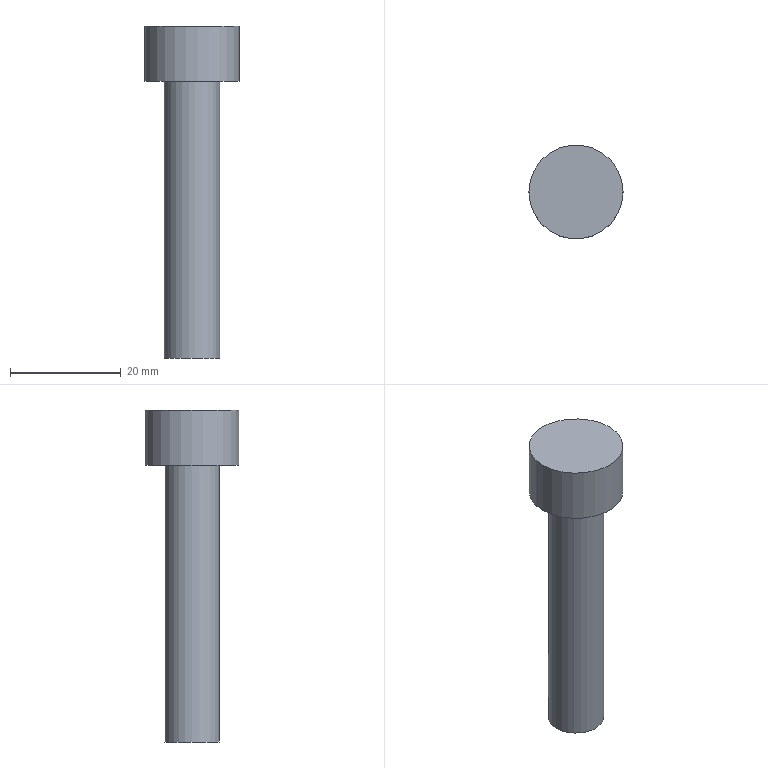Part | NX | features solid 2 | 1 solid | 5 faces | box 17 x 17 x 60 mm | volume 6197 mm3 | plane 3 | cylinder 2 | commonest cylinder face diameters 10 x1 17 x1
STEP:
#1=CARTESIAN_POINT('',(-5.,447.,-123.));
#2=VERTEX_POINT('',#1);
#3=CARTESIAN_POINT('',(0.,447.,-123.));
#4=DIRECTION('',(0.,0.,-1.));
#5=DIRECTION('',(-1.,0.,0.));
#6=AXIS2_PLACEMENT_3D('',#3,#4,#5);
#7=CIRCLE('',#6,5.);
#8=EDGE_CURVE('',#2,#2,#7,.T.);
#9=ORIENTED_EDGE('',*,*,#8,.T.);
#10=EDGE_LOOP('',(#9));
#11=FACE_BOUND('',#10,.T.);
#12=CARTESIAN_POINT('',(0.,447.,-123.));
#13=DIRECTION('',(0.,0.,-1.));
#14=DIRECTION('',(-1.,0.,0.));
#15=AXIS2_PLACEMENT_3D('',#12,#13,#14);
#16=PLANE('',#15);
#17=ADVANCED_FACE('',(#11),#16,.T.);
#18=CARTESIAN_POINT('',(-5.,447.,-73.));
#19=VERTEX_POINT('',#18);
#20=CARTESIAN_POINT('',(0.,447.,-73.));
#21=DIRECTION('',(0.,0.,-1.));
#22=DIRECTION('',(-1.,0.,0.));
#23=AXIS2_PLACEMENT_3D('',#20,#21,#22);
#24=CIRCLE('',#23,5.);
#25=EDGE_CURVE('',#19,#19,#24,.F.);
#26=ORIENTED_EDGE('',*,*,#25,.F.);
#27=EDGE_LOOP('',(#26));
#28=FACE_BOUND('',#27,.T.);
#29=ORIENTED_EDGE('',*,*,#8,.F.);
#30=EDGE_LOOP('',(#29));
#31=FACE_BOUND('',#30,.T.);
#32=CARTESIAN_POINT('',(0.,447.,-83.));
#33=DIRECTION('',(0.,0.,-1.));
#34=DIRECTION('',(-1.,0.,0.));
#35=AXIS2_PLACEMENT_3D('',#32,#33,#34);
#36=CYLINDRICAL_SURFACE('',#35,5.);
#37=ADVANCED_FACE('',(#28,#31),#36,.T.);
#38=CARTESIAN_POINT('',(-8.5,447.,-63.));
#39=VERTEX_POINT('',#38);
#40=CARTESIAN_POINT('',(0.,447.,-63.));
#41=DIRECTION('',(0.,0.,-1.));
#42=DIRECTION('',(-1.,0.,0.));
#43=AXIS2_PLACEMENT_3D('',#40,#41,#42);
#44=CIRCLE('',#43,8.5);
#45=EDGE_CURVE('',#39,#39,#44,.F.);
#46=ORIENTED_EDGE('',*,*,#45,.F.);
#47=EDGE_LOOP('',(#46));
#48=FACE_BOUND('',#47,.T.);
#49=CARTESIAN_POINT('',(-8.5,447.,-73.));
#50=VERTEX_POINT('',#49);
#51=CARTESIAN_POINT('',(0.,447.,-73.));
#52=DIRECTION('',(0.,0.,-1.));
#53=DIRECTION('',(-1.,0.,0.));
#54=AXIS2_PLACEMENT_3D('',#51,#52,#53);
#55=CIRCLE('',#54,8.5);
#56=EDGE_CURVE('',#50,#50,#55,.F.);
#57=ORIENTED_EDGE('',*,*,#56,.T.);
#58=EDGE_LOOP('',(#57));
#59=FACE_BOUND('',#58,.T.);
#60=CARTESIAN_POINT('',(0.,447.,-73.));
#61=DIRECTION('',(0.,0.,1.));
#62=DIRECTION('',(1.,0.,0.));
#63=AXIS2_PLACEMENT_3D('',#60,#61,#62);
#64=CYLINDRICAL_SURFACE('',#63,8.5);
#65=ADVANCED_FACE('',(#48,#59),#64,.T.);
#66=ORIENTED_EDGE('',*,*,#56,.F.);
#67=EDGE_LOOP('',(#66));
#68=FACE_BOUND('',#67,.T.);
#69=ORIENTED_EDGE('',*,*,#25,.T.);
#70=EDGE_LOOP('',(#69));
#71=FACE_BOUND('',#70,.T.);
#72=CARTESIAN_POINT('',(0.,447.,-73.));
#73=DIRECTION('',(0.,0.,-1.));
#74=DIRECTION('',(-1.,0.,0.));
#75=AXIS2_PLACEMENT_3D('',#72,#73,#74);
#76=PLANE('',#75);
#77=ADVANCED_FACE('',(#68,#71),#76,.T.);
#78=ORIENTED_EDGE('',*,*,#45,.T.);
#79=EDGE_LOOP('',(#78));
#80=FACE_BOUND('',#79,.T.);
#81=CARTESIAN_POINT('',(0.,447.,-63.));
#82=DIRECTION('',(0.,0.,-1.));
#83=DIRECTION('',(-1.,0.,0.));
#84=AXIS2_PLACEMENT_3D('',#81,#82,#83);
#85=PLANE('',#84);
#86=ADVANCED_FACE('',(#80),#85,.F.);
#87=CLOSED_SHELL('',(#17,#37,#65,#77,#86));
#88=MANIFOLD_SOLID_BREP('',#87);
#89=(LENGTH_UNIT()NAMED_UNIT(*)SI_UNIT(.MILLI.,.METRE.));
#90=UNCERTAINTY_MEASURE_WITH_UNIT(LENGTH_MEASURE(0.00001),#89,'','');
#91=(NAMED_UNIT(*)PLANE_ANGLE_UNIT()SI_UNIT($,.RADIAN.));
#92=(NAMED_UNIT(*)SI_UNIT($,.STERADIAN.)SOLID_ANGLE_UNIT());
#93=(GEOMETRIC_REPRESENTATION_CONTEXT(3)GLOBAL_UNCERTAINTY_ASSIGNED_CONTEXT((#90))GLOBAL_UNIT_ASSIGNED_CONTEXT((#89,#91,#92))REPRESENTATION_CONTEXT('',''));
#94=ADVANCED_BREP_SHAPE_REPRESENTATION('',(#88),#93);